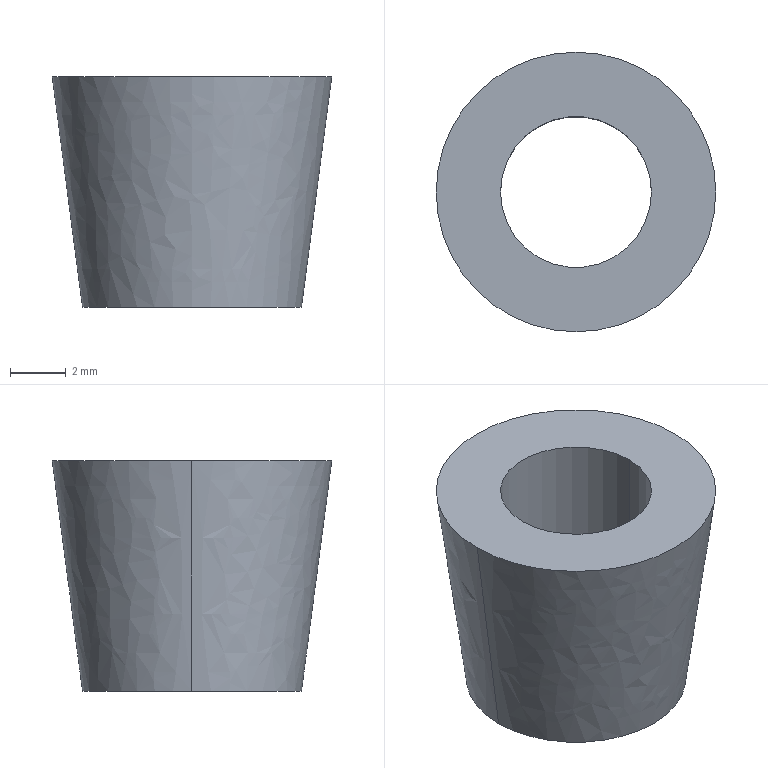Part | SolidWorks | features Blend 1, ICE 1 | 1 solid | 6 faces | box 10 x 10 x 8.25 mm | volume 327.849 mm3 | cylinder 2 | spline 2 | plane 2 | commonest cylinder face diameters 5.4 x2
STEP:
#1=CARTESIAN_POINT('',(2.7,0.,8.25));
#2=VERTEX_POINT('',#1);
#3=CARTESIAN_POINT('',(-2.7,0.,8.25));
#4=VERTEX_POINT('',#3);
#5=CARTESIAN_POINT('',(0.,0.,8.25));
#6=DIRECTION('',(0.,0.,-1.));
#7=DIRECTION('',(1.,0.,0.));
#8=AXIS2_PLACEMENT_3D('',#5,#6,#7);
#9=CIRCLE('',#8,2.7);
#10=EDGE_CURVE('',#2,#4,#9,.T.);
#11=ORIENTED_EDGE('',*,*,#10,.F.);
#12=CARTESIAN_POINT('',(2.7,0.,0.));
#13=VERTEX_POINT('',#12);
#14=CARTESIAN_POINT('',(2.7,0.,8.263));
#15=DIRECTION('',(0.,0.,-1.));
#16=VECTOR('',#15,1000.);
#17=LINE('',#14,#16);
#18=EDGE_CURVE('',#2,#13,#17,.T.);
#19=ORIENTED_EDGE('',*,*,#18,.T.);
#20=CARTESIAN_POINT('',(-2.7,0.,0.));
#21=VERTEX_POINT('',#20);
#22=CARTESIAN_POINT('',(0.,0.,0.));
#23=DIRECTION('',(0.,0.,-1.));
#24=DIRECTION('',(-1.,0.,0.));
#25=AXIS2_PLACEMENT_3D('',#22,#23,#24);
#26=CIRCLE('',#25,2.7);
#27=EDGE_CURVE('',#13,#21,#26,.T.);
#28=ORIENTED_EDGE('',*,*,#27,.T.);
#29=CARTESIAN_POINT('',(-2.7,0.,8.263));
#30=DIRECTION('',(0.,0.,-1.));
#31=VECTOR('',#30,1000.);
#32=LINE('',#29,#31);
#33=EDGE_CURVE('',#4,#21,#32,.T.);
#34=ORIENTED_EDGE('',*,*,#33,.F.);
#35=EDGE_LOOP('',(#11,#19,#28,#34));
#36=FACE_OUTER_BOUND('',#35,.T.);
#37=CARTESIAN_POINT('',(0.,0.,8.263));
#38=DIRECTION('',(0.,0.,-1.));
#39=DIRECTION('',(-1.,0.,0.));
#40=AXIS2_PLACEMENT_3D('',#37,#38,#39);
#41=CYLINDRICAL_SURFACE('',#40,2.7);
#42=ADVANCED_FACE('',(#36),#41,.F.);
#43=CARTESIAN_POINT('',(-3.915,0.,0.));
#44=VERTEX_POINT('',#43);
#45=CARTESIAN_POINT('',(3.915,0.,0.));
#46=VERTEX_POINT('',#45);
#47=CARTESIAN_POINT('',(0.,0.,0.));
#48=DIRECTION('',(0.,0.,1.));
#49=DIRECTION('',(1.,0.,0.));
#50=AXIS2_PLACEMENT_3D('',#47,#48,#49);
#51=CIRCLE('',#50,3.915);
#52=EDGE_CURVE('',#44,#46,#51,.T.);
#53=ORIENTED_EDGE('',*,*,#52,.T.);
#54=CARTESIAN_POINT('',(5.,0.,8.25));
#55=VERTEX_POINT('',#54);
#56=CARTESIAN_POINT('',(3.915,0.,0.));
#57=CARTESIAN_POINT('',(4.277,0.,2.75));
#58=CARTESIAN_POINT('',(4.638,0.,5.5));
#59=CARTESIAN_POINT('',(5.,0.,8.25));
#60=B_SPLINE_CURVE_WITH_KNOTS('',3,(#56,#57,#58,#59),.UNSPECIFIED.,.F.,.F.,(4,4),(0.,1.),.UNSPECIFIED.);
#61=EDGE_CURVE('',#46,#55,#60,.T.);
#62=ORIENTED_EDGE('',*,*,#61,.T.);
#63=CARTESIAN_POINT('',(-5.,0.,8.25));
#64=VERTEX_POINT('',#63);
#65=CARTESIAN_POINT('',(0.,0.,8.25));
#66=DIRECTION('',(0.,0.,1.));
#67=DIRECTION('',(1.,0.,0.));
#68=AXIS2_PLACEMENT_3D('',#65,#66,#67);
#69=CIRCLE('',#68,5.);
#70=EDGE_CURVE('',#64,#55,#69,.T.);
#71=ORIENTED_EDGE('',*,*,#70,.F.);
#72=CARTESIAN_POINT('',(-3.915,0.,0.));
#73=CARTESIAN_POINT('',(-4.277,0.,2.75));
#74=CARTESIAN_POINT('',(-4.638,0.,5.5));
#75=CARTESIAN_POINT('',(-5.,0.,8.25));
#76=B_SPLINE_CURVE_WITH_KNOTS('',3,(#72,#73,#74,#75),.UNSPECIFIED.,.F.,.F.,(4,4),(0.,1.),.UNSPECIFIED.);
#77=EDGE_CURVE('',#44,#64,#76,.T.);
#78=ORIENTED_EDGE('',*,*,#77,.F.);
#79=EDGE_LOOP('',(#53,#62,#71,#78));
#80=FACE_OUTER_BOUND('',#79,.T.);
#81=CARTESIAN_POINT('',(-3.915,0.,0.));
#82=CARTESIAN_POINT('',(-4.277,0.,2.75));
#83=CARTESIAN_POINT('',(-4.638,0.,5.5));
#84=CARTESIAN_POINT('',(-5.,0.,8.25));
#85=CARTESIAN_POINT('',(-3.915,-0.108,0.));
#86=CARTESIAN_POINT('',(-4.277,-0.118,2.75));
#87=CARTESIAN_POINT('',(-4.638,-0.128,5.5));
#88=CARTESIAN_POINT('',(-5.,-0.138,8.25));
#89=CARTESIAN_POINT('',(-3.906,-0.3221,0.));
#90=CARTESIAN_POINT('',(-4.267,-0.3518,2.75));
#91=CARTESIAN_POINT('',(-4.628,-0.3816,5.5));
#92=CARTESIAN_POINT('',(-4.989,-0.4113,8.25));
#93=CARTESIAN_POINT('',(-3.868,-0.636,0.));
#94=CARTESIAN_POINT('',(-4.225,-0.6948,2.75));
#95=CARTESIAN_POINT('',(-4.582,-0.7535,5.5));
#96=CARTESIAN_POINT('',(-4.94,-0.8123,8.25));
#97=CARTESIAN_POINT('',(-3.805,-0.9419,0.));
#98=CARTESIAN_POINT('',(-4.157,-1.029,2.75));
#99=CARTESIAN_POINT('',(-4.508,-1.116,5.5));
#100=CARTESIAN_POINT('',(-4.86,-1.203,8.25));
#101=CARTESIAN_POINT('',(-3.289,-2.722,0.));
#102=CARTESIAN_POINT('',(-3.593,-2.974,2.75));
#103=CARTESIAN_POINT('',(-3.896,-3.225,5.5));
#104=CARTESIAN_POINT('',(-4.2,-3.477,8.25));
#105=CARTESIAN_POINT('',(-1.729,-3.915,0.));
#106=CARTESIAN_POINT('',(-1.888,-4.277,2.75));
#107=CARTESIAN_POINT('',(-2.048,-4.638,5.5));
#108=CARTESIAN_POINT('',(-2.208,-5.,8.25));
#109=CARTESIAN_POINT('',(2.161,-3.915,0.));
#110=CARTESIAN_POINT('',(2.36,-4.277,2.75));
#111=CARTESIAN_POINT('',(2.56,-4.638,5.5));
#112=CARTESIAN_POINT('',(2.76,-5.,8.25));
#113=CARTESIAN_POINT('',(3.915,-2.161,0.));
#114=CARTESIAN_POINT('',(4.277,-2.36,2.75));
#115=CARTESIAN_POINT('',(4.638,-2.56,5.5));
#116=CARTESIAN_POINT('',(5.,-2.76,8.25));
#117=CARTESIAN_POINT('',(3.915,2.161,0.));
#118=CARTESIAN_POINT('',(4.277,2.36,2.75));
#119=CARTESIAN_POINT('',(4.638,2.56,5.5));
#120=CARTESIAN_POINT('',(5.,2.76,8.25));
#121=CARTESIAN_POINT('',(2.161,3.915,0.));
#122=CARTESIAN_POINT('',(2.36,4.277,2.75));
#123=CARTESIAN_POINT('',(2.56,4.638,5.5));
#124=CARTESIAN_POINT('',(2.76,5.,8.25));
#125=CARTESIAN_POINT('',(-1.729,3.915,0.));
#126=CARTESIAN_POINT('',(-1.888,4.277,2.75));
#127=CARTESIAN_POINT('',(-2.048,4.638,5.5));
#128=CARTESIAN_POINT('',(-2.208,5.,8.25));
#129=CARTESIAN_POINT('',(-3.289,2.722,0.));
#130=CARTESIAN_POINT('',(-3.593,2.974,2.75));
#131=CARTESIAN_POINT('',(-3.896,3.225,5.5));
#132=CARTESIAN_POINT('',(-4.2,3.477,8.25));
#133=CARTESIAN_POINT('',(-3.805,0.9419,0.));
#134=CARTESIAN_POINT('',(-4.157,1.029,2.75));
#135=CARTESIAN_POINT('',(-4.508,1.116,5.5));
#136=CARTESIAN_POINT('',(-4.86,1.203,8.25));
#137=CARTESIAN_POINT('',(-3.868,0.636,0.));
#138=CARTESIAN_POINT('',(-4.225,0.6948,2.75));
#139=CARTESIAN_POINT('',(-4.582,0.7535,5.5));
#140=CARTESIAN_POINT('',(-4.94,0.8123,8.25));
#141=CARTESIAN_POINT('',(-3.906,0.3221,0.));
#142=CARTESIAN_POINT('',(-4.267,0.3518,2.75));
#143=CARTESIAN_POINT('',(-4.628,0.3816,5.5));
#144=CARTESIAN_POINT('',(-4.989,0.4113,8.25));
#145=CARTESIAN_POINT('',(-3.915,0.108,0.));
#146=CARTESIAN_POINT('',(-4.277,0.118,2.75));
#147=CARTESIAN_POINT('',(-4.638,0.128,5.5));
#148=CARTESIAN_POINT('',(-5.,0.138,8.25));
#149=CARTESIAN_POINT('',(-3.915,0.,0.));
#150=CARTESIAN_POINT('',(-4.277,0.,2.75));
#151=CARTESIAN_POINT('',(-4.638,0.,5.5));
#152=CARTESIAN_POINT('',(-5.,0.,8.25));
#153=B_SPLINE_SURFACE_WITH_KNOTS('',3,3,((#81,#82,#83,#84),(#85,#86,#87,#88),(#89,#90,#91,#92),(#93,#94,#95,#96),(#97,#98,#99,#100),(#101,#102,#103,#104),(#105,#106,#107,#108),(#109,#110,#111,#112),(#113,#114,#115,#116),(#117,#118,#119,#120),(#121,#122,#123,#124),(#125,#126,#127,#128),(#129,#130,#131,#132),(#133,#134,#135,#136),(#137,#138,#139,#140),(#141,#142,#143,#144),(#145,#146,#147,#148),(#149,#150,#151,#152)),.UNSPECIFIED.,.T.,.F.,.F.,(4,1,1,1,1,2,2,2,1,1,1,1,4),(4,4),(0.,0.0125,0.025,0.0375,0.05,0.25,0.5,0.75,0.95,0.9625,0.975,0.9875,1.),(0.,1.),.UNSPECIFIED.);
#154=ADVANCED_FACE('',(#80),#153,.T.);
#155=CARTESIAN_POINT('',(0.,0.,8.25));
#156=DIRECTION('',(0.,0.,-1.));
#157=DIRECTION('',(1.,0.,0.));
#158=AXIS2_PLACEMENT_3D('',#155,#156,#157);
#159=CIRCLE('',#158,2.7);
#160=EDGE_CURVE('',#4,#2,#159,.T.);
#161=ORIENTED_EDGE('',*,*,#160,.T.);
#162=ORIENTED_EDGE('',*,*,#10,.T.);
#163=EDGE_LOOP('',(#161,#162));
#164=FACE_BOUND('',#163,.T.);
#165=ORIENTED_EDGE('',*,*,#70,.T.);
#166=CARTESIAN_POINT('',(0.,0.,8.25));
#167=DIRECTION('',(0.,0.,1.));
#168=DIRECTION('',(1.,0.,0.));
#169=AXIS2_PLACEMENT_3D('',#166,#167,#168);
#170=CIRCLE('',#169,5.);
#171=EDGE_CURVE('',#55,#64,#170,.T.);
#172=ORIENTED_EDGE('',*,*,#171,.T.);
#173=EDGE_LOOP('',(#165,#172));
#174=FACE_OUTER_BOUND('',#173,.T.);
#175=CARTESIAN_POINT('',(0.,0.,8.25));
#176=DIRECTION('',(0.,0.,1.));
#177=DIRECTION('',(1.,0.,0.));
#178=AXIS2_PLACEMENT_3D('',#175,#176,#177);
#179=PLANE('',#178);
#180=ADVANCED_FACE('',(#164,#174),#179,.T.);
#181=CARTESIAN_POINT('',(0.,0.,0.));
#182=DIRECTION('',(0.,0.,-1.));
#183=DIRECTION('',(-1.,0.,0.));
#184=AXIS2_PLACEMENT_3D('',#181,#182,#183);
#185=CIRCLE('',#184,2.7);
#186=EDGE_CURVE('',#21,#13,#185,.T.);
#187=ORIENTED_EDGE('',*,*,#186,.F.);
#188=ORIENTED_EDGE('',*,*,#27,.F.);
#189=EDGE_LOOP('',(#187,#188));
#190=FACE_BOUND('',#189,.T.);
#191=ORIENTED_EDGE('',*,*,#52,.F.);
#192=CARTESIAN_POINT('',(0.,0.,0.));
#193=DIRECTION('',(0.,0.,1.));
#194=DIRECTION('',(1.,0.,0.));
#195=AXIS2_PLACEMENT_3D('',#192,#193,#194);
#196=CIRCLE('',#195,3.915);
#197=EDGE_CURVE('',#46,#44,#196,.T.);
#198=ORIENTED_EDGE('',*,*,#197,.F.);
#199=EDGE_LOOP('',(#191,#198));
#200=FACE_OUTER_BOUND('',#199,.T.);
#201=CARTESIAN_POINT('',(0.,0.,0.));
#202=DIRECTION('',(0.,0.,1.));
#203=DIRECTION('',(1.,0.,0.));
#204=AXIS2_PLACEMENT_3D('',#201,#202,#203);
#205=PLANE('',#204);
#206=ADVANCED_FACE('',(#190,#200),#205,.F.);
#207=ORIENTED_EDGE('',*,*,#61,.F.);
#208=ORIENTED_EDGE('',*,*,#197,.T.);
#209=ORIENTED_EDGE('',*,*,#77,.T.);
#210=ORIENTED_EDGE('',*,*,#171,.F.);
#211=EDGE_LOOP('',(#207,#208,#209,#210));
#212=FACE_OUTER_BOUND('',#211,.T.);
#213=CARTESIAN_POINT('',(-3.915,0.,0.));
#214=CARTESIAN_POINT('',(-4.277,0.,2.75));
#215=CARTESIAN_POINT('',(-4.638,0.,5.5));
#216=CARTESIAN_POINT('',(-5.,0.,8.25));
#217=CARTESIAN_POINT('',(-3.915,-0.108,0.));
#218=CARTESIAN_POINT('',(-4.277,-0.118,2.75));
#219=CARTESIAN_POINT('',(-4.638,-0.128,5.5));
#220=CARTESIAN_POINT('',(-5.,-0.138,8.25));
#221=CARTESIAN_POINT('',(-3.906,-0.3221,0.));
#222=CARTESIAN_POINT('',(-4.267,-0.3518,2.75));
#223=CARTESIAN_POINT('',(-4.628,-0.3816,5.5));
#224=CARTESIAN_POINT('',(-4.989,-0.4113,8.25));
#225=CARTESIAN_POINT('',(-3.868,-0.636,0.));
#226=CARTESIAN_POINT('',(-4.225,-0.6948,2.75));
#227=CARTESIAN_POINT('',(-4.582,-0.7535,5.5));
#228=CARTESIAN_POINT('',(-4.94,-0.8123,8.25));
#229=CARTESIAN_POINT('',(-3.805,-0.9419,0.));
#230=CARTESIAN_POINT('',(-4.157,-1.029,2.75));
#231=CARTESIAN_POINT('',(-4.508,-1.116,5.5));
#232=CARTESIAN_POINT('',(-4.86,-1.203,8.25));
#233=CARTESIAN_POINT('',(-3.289,-2.722,0.));
#234=CARTESIAN_POINT('',(-3.593,-2.974,2.75));
#235=CARTESIAN_POINT('',(-3.896,-3.225,5.5));
#236=CARTESIAN_POINT('',(-4.2,-3.477,8.25));
#237=CARTESIAN_POINT('',(-1.729,-3.915,0.));
#238=CARTESIAN_POINT('',(-1.888,-4.277,2.75));
#239=CARTESIAN_POINT('',(-2.048,-4.638,5.5));
#240=CARTESIAN_POINT('',(-2.208,-5.,8.25));
#241=CARTESIAN_POINT('',(2.161,-3.915,0.));
#242=CARTESIAN_POINT('',(2.36,-4.277,2.75));
#243=CARTESIAN_POINT('',(2.56,-4.638,5.5));
#244=CARTESIAN_POINT('',(2.76,-5.,8.25));
#245=CARTESIAN_POINT('',(3.915,-2.161,0.));
#246=CARTESIAN_POINT('',(4.277,-2.36,2.75));
#247=CARTESIAN_POINT('',(4.638,-2.56,5.5));
#248=CARTESIAN_POINT('',(5.,-2.76,8.25));
#249=CARTESIAN_POINT('',(3.915,2.161,0.));
#250=CARTESIAN_POINT('',(4.277,2.36,2.75));
#251=CARTESIAN_POINT('',(4.638,2.56,5.5));
#252=CARTESIAN_POINT('',(5.,2.76,8.25));
#253=CARTESIAN_POINT('',(2.161,3.915,0.));
#254=CARTESIAN_POINT('',(2.36,4.277,2.75));
#255=CARTESIAN_POINT('',(2.56,4.638,5.5));
#256=CARTESIAN_POINT('',(2.76,5.,8.25));
#257=CARTESIAN_POINT('',(-1.729,3.915,0.));
#258=CARTESIAN_POINT('',(-1.888,4.277,2.75));
#259=CARTESIAN_POINT('',(-2.048,4.638,5.5));
#260=CARTESIAN_POINT('',(-2.208,5.,8.25));
#261=CARTESIAN_POINT('',(-3.289,2.722,0.));
#262=CARTESIAN_POINT('',(-3.593,2.974,2.75));
#263=CARTESIAN_POINT('',(-3.896,3.225,5.5));
#264=CARTESIAN_POINT('',(-4.2,3.477,8.25));
#265=CARTESIAN_POINT('',(-3.805,0.9419,0.));
#266=CARTESIAN_POINT('',(-4.157,1.029,2.75));
#267=CARTESIAN_POINT('',(-4.508,1.116,5.5));
#268=CARTESIAN_POINT('',(-4.86,1.203,8.25));
#269=CARTESIAN_POINT('',(-3.868,0.636,0.));
#270=CARTESIAN_POINT('',(-4.225,0.6948,2.75));
#271=CARTESIAN_POINT('',(-4.582,0.7535,5.5));
#272=CARTESIAN_POINT('',(-4.94,0.8123,8.25));
#273=CARTESIAN_POINT('',(-3.906,0.3221,0.));
#274=CARTESIAN_POINT('',(-4.267,0.3518,2.75));
#275=CARTESIAN_POINT('',(-4.628,0.3816,5.5));
#276=CARTESIAN_POINT('',(-4.989,0.4113,8.25));
#277=CARTESIAN_POINT('',(-3.915,0.108,0.));
#278=CARTESIAN_POINT('',(-4.277,0.118,2.75));
#279=CARTESIAN_POINT('',(-4.638,0.128,5.5));
#280=CARTESIAN_POINT('',(-5.,0.138,8.25));
#281=CARTESIAN_POINT('',(-3.915,0.,0.));
#282=CARTESIAN_POINT('',(-4.277,0.,2.75));
#283=CARTESIAN_POINT('',(-4.638,0.,5.5));
#284=CARTESIAN_POINT('',(-5.,0.,8.25));
#285=B_SPLINE_SURFACE_WITH_KNOTS('',3,3,((#213,#214,#215,#216),(#217,#218,#219,#220),(#221,#222,#223,#224),(#225,#226,#227,#228),(#229,#230,#231,#232),(#233,#234,#235,#236),(#237,#238,#239,#240),(#241,#242,#243,#244),(#245,#246,#247,#248),(#249,#250,#251,#252),(#253,#254,#255,#256),(#257,#258,#259,#260),(#261,#262,#263,#264),(#265,#266,#267,#268),(#269,#270,#271,#272),(#273,#274,#275,#276),(#277,#278,#279,#280),(#281,#282,#283,#284)),.UNSPECIFIED.,.T.,.F.,.F.,(4,1,1,1,1,2,2,2,1,1,1,1,4),(4,4),(0.,0.0125,0.025,0.0375,0.05,0.25,0.5,0.75,0.95,0.9625,0.975,0.9875,1.),(0.,1.),.UNSPECIFIED.);
#286=ADVANCED_FACE('',(#212),#285,.T.);
#287=ORIENTED_EDGE('',*,*,#18,.F.);
#288=ORIENTED_EDGE('',*,*,#160,.F.);
#289=ORIENTED_EDGE('',*,*,#33,.T.);
#290=ORIENTED_EDGE('',*,*,#186,.T.);
#291=EDGE_LOOP('',(#287,#288,#289,#290));
#292=FACE_OUTER_BOUND('',#291,.T.);
#293=CARTESIAN_POINT('',(0.,0.,8.263));
#294=DIRECTION('',(0.,0.,-1.));
#295=DIRECTION('',(-1.,0.,0.));
#296=AXIS2_PLACEMENT_3D('',#293,#294,#295);
#297=CYLINDRICAL_SURFACE('',#296,2.7);
#298=ADVANCED_FACE('',(#292),#297,.F.);
#299=CLOSED_SHELL('',(#42,#154,#180,#206,#286,#298));
#300=MANIFOLD_SOLID_BREP('',#299);
#301=CARTESIAN_POINT('',(0.,0.,0.));
#302=DIRECTION('',(0.,0.,1.));
#303=DIRECTION('',(1.,0.,0.));
#304=AXIS2_PLACEMENT_3D('',#301,#302,#303);
#305=(LENGTH_UNIT()NAMED_UNIT(*)SI_UNIT(.MILLI.,.METRE.));
#306=UNCERTAINTY_MEASURE_WITH_UNIT(LENGTH_MEASURE(0.00001),#305,'','');
#307=(NAMED_UNIT(*)PLANE_ANGLE_UNIT()SI_UNIT($,.RADIAN.));
#308=(NAMED_UNIT(*)SI_UNIT($,.STERADIAN.)SOLID_ANGLE_UNIT());
#309=(GEOMETRIC_REPRESENTATION_CONTEXT(3)GLOBAL_UNCERTAINTY_ASSIGNED_CONTEXT((#306))GLOBAL_UNIT_ASSIGNED_CONTEXT((#305,#307,#308))REPRESENTATION_CONTEXT('',''));
#310=ADVANCED_BREP_SHAPE_REPRESENTATION('',(#300,#304),#309);